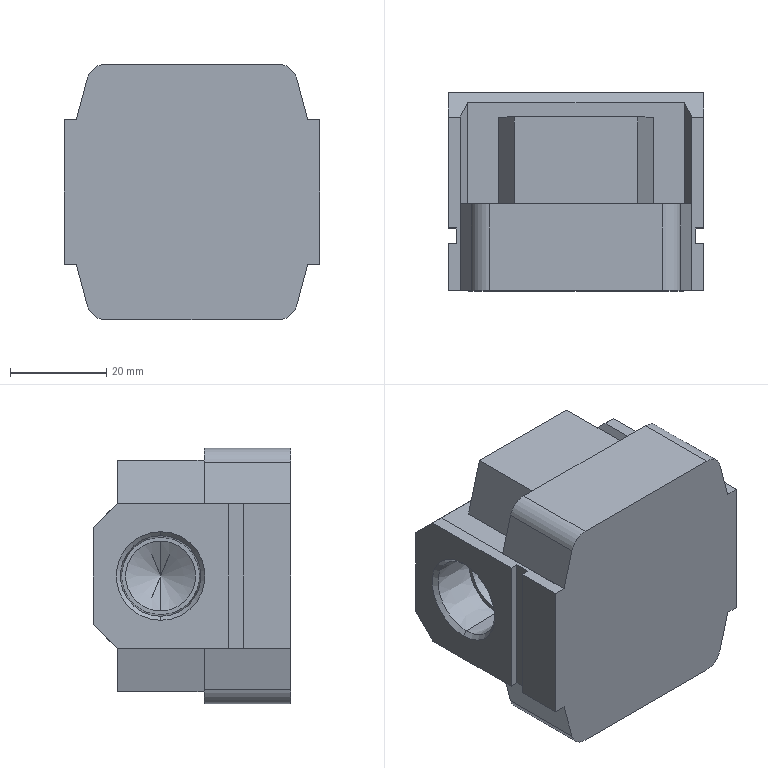Part | STEP file | AFM30-03_AFM3022A Body_30 | 1 solid | 102 faces | box 53 x 41 x 53 mm | volume 82463 mm3 | plane 50 | cone 28 | cylinder 24 | commonest cylinder face diameters 3.3 x8 4 x8 8 x4 14.5 x4